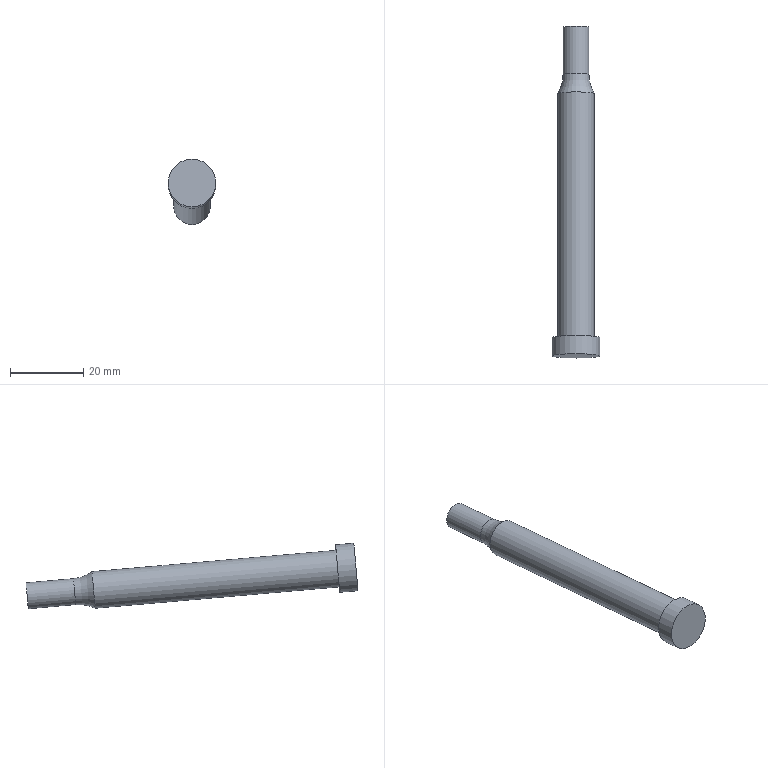Part | NX | features SPAS 10-80-7.100 2 | 1 solid | 7 faces | box 13 x 90.533 x 17.856 mm | volume 6692 mm3 | plane 3 | cylinder 3 | torus 1 | commonest cylinder face diameters 7.1 x1 10 x1 13 x1
STEP:
#1=CARTESIAN_POINT('',(-242.835,-53.602,-36.764));
#2=VERTEX_POINT('',#1);
#3=CARTESIAN_POINT('',(-242.835,-53.292,-33.227));
#4=DIRECTION('',(0.,-0.9962,0.08716));
#5=DIRECTION('',(0.,-0.08716,-0.9962));
#6=AXIS2_PLACEMENT_3D('',#3,#4,#5);
#7=CIRCLE('',#6,3.55);
#8=EDGE_CURVE('',#2,#2,#7,.T.);
#9=ORIENTED_EDGE('',*,*,#8,.F.);
#10=EDGE_LOOP('',(#9));
#11=FACE_BOUND('',#10,.T.);
#12=CARTESIAN_POINT('',(-242.835,-53.292,-33.227));
#13=DIRECTION('',(0.,0.9962,-0.08716));
#14=DIRECTION('',(0.,0.08716,0.9962));
#15=AXIS2_PLACEMENT_3D('',#12,#13,#14);
#16=PLANE('',#15);
#17=ADVANCED_FACE('',(#11),#16,.T.);
#18=CARTESIAN_POINT('',(-242.835,-66.552,-35.631));
#19=VERTEX_POINT('',#18);
#20=CARTESIAN_POINT('',(-242.835,-66.243,-32.094));
#21=DIRECTION('',(0.,-0.9962,0.08716));
#22=DIRECTION('',(0.,-0.08716,-0.9962));
#23=AXIS2_PLACEMENT_3D('',#20,#21,#22);
#24=CIRCLE('',#23,3.55);
#25=EDGE_CURVE('',#19,#19,#24,.F.);
#26=ORIENTED_EDGE('',*,*,#25,.T.);
#27=EDGE_LOOP('',(#26));
#28=FACE_BOUND('',#27,.T.);
#29=ORIENTED_EDGE('',*,*,#8,.T.);
#30=EDGE_LOOP('',(#29));
#31=FACE_BOUND('',#30,.T.);
#32=CARTESIAN_POINT('',(-242.835,-53.292,-33.227));
#33=DIRECTION('',(0.,-0.9962,0.08716));
#34=DIRECTION('',(0.,-0.08716,-0.9962));
#35=AXIS2_PLACEMENT_3D('',#32,#33,#34);
#36=CYLINDRICAL_SURFACE('',#35,3.55);
#37=ADVANCED_FACE('',(#28,#31),#36,.T.);
#38=CARTESIAN_POINT('',(-242.835,-137.533,-20.838));
#39=VERTEX_POINT('',#38);
#40=CARTESIAN_POINT('',(-242.835,-137.969,-25.819));
#41=DIRECTION('',(0.,0.9962,-0.08716));
#42=DIRECTION('',(0.,0.08716,0.9962));
#43=AXIS2_PLACEMENT_3D('',#40,#41,#42);
#44=CIRCLE('',#43,5.);
#45=EDGE_CURVE('',#39,#39,#44,.F.);
#46=ORIENTED_EDGE('',*,*,#45,.F.);
#47=EDGE_LOOP('',(#46));
#48=FACE_BOUND('',#47,.T.);
#49=CARTESIAN_POINT('',(-242.835,-71.845,-36.623));
#50=VERTEX_POINT('',#49);
#51=CARTESIAN_POINT('',(-242.835,-71.409,-31.642));
#52=DIRECTION('',(0.,-0.9962,0.08716));
#53=DIRECTION('',(0.,-0.08716,-0.9962));
#54=AXIS2_PLACEMENT_3D('',#51,#52,#53);
#55=CIRCLE('',#54,5.);
#56=EDGE_CURVE('',#50,#50,#55,.T.);
#57=ORIENTED_EDGE('',*,*,#56,.T.);
#58=EDGE_LOOP('',(#57));
#59=FACE_BOUND('',#58,.T.);
#60=CARTESIAN_POINT('',(-242.835,-71.409,-31.642));
#61=DIRECTION('',(0.,-0.9962,0.08716));
#62=DIRECTION('',(0.,-0.08716,-0.9962));
#63=AXIS2_PLACEMENT_3D('',#60,#61,#62);
#64=CYLINDRICAL_SURFACE('',#63,5.);
#65=ADVANCED_FACE('',(#48,#59),#64,.T.);
#66=CARTESIAN_POINT('',(-242.835,-143.516,-31.859));
#67=VERTEX_POINT('',#66);
#68=CARTESIAN_POINT('',(-242.835,-142.95,-25.383));
#69=DIRECTION('',(0.,-0.9962,0.08716));
#70=DIRECTION('',(0.,-0.08716,-0.9962));
#71=AXIS2_PLACEMENT_3D('',#68,#69,#70);
#72=CIRCLE('',#71,6.5);
#73=EDGE_CURVE('',#67,#67,#72,.F.);
#74=ORIENTED_EDGE('',*,*,#73,.F.);
#75=EDGE_LOOP('',(#74));
#76=FACE_BOUND('',#75,.T.);
#77=CARTESIAN_POINT('',(-242.835,-142.95,-25.383));
#78=DIRECTION('',(0.,-0.9962,0.08716));
#79=DIRECTION('',(0.,-0.08716,-0.9962));
#80=AXIS2_PLACEMENT_3D('',#77,#78,#79);
#81=PLANE('',#80);
#82=ADVANCED_FACE('',(#76),#81,.T.);
#83=ORIENTED_EDGE('',*,*,#45,.T.);
#84=EDGE_LOOP('',(#83));
#85=FACE_BOUND('',#84,.T.);
#86=CARTESIAN_POINT('',(-242.835,-137.402,-19.344));
#87=VERTEX_POINT('',#86);
#88=CARTESIAN_POINT('',(-242.835,-137.969,-25.819));
#89=DIRECTION('',(0.,0.9962,-0.08716));
#90=DIRECTION('',(0.,0.08716,0.9962));
#91=AXIS2_PLACEMENT_3D('',#88,#89,#90);
#92=CIRCLE('',#91,6.5);
#93=EDGE_CURVE('',#87,#87,#92,.F.);
#94=ORIENTED_EDGE('',*,*,#93,.F.);
#95=EDGE_LOOP('',(#94));
#96=FACE_BOUND('',#95,.T.);
#97=CARTESIAN_POINT('',(-242.835,-137.969,-25.819));
#98=DIRECTION('',(0.,0.9962,-0.08716));
#99=DIRECTION('',(0.,0.08716,0.9962));
#100=AXIS2_PLACEMENT_3D('',#97,#98,#99);
#101=PLANE('',#100);
#102=ADVANCED_FACE('',(#85,#96),#101,.T.);
#103=ORIENTED_EDGE('',*,*,#73,.T.);
#104=EDGE_LOOP('',(#103));
#105=FACE_BOUND('',#104,.T.);
#106=ORIENTED_EDGE('',*,*,#93,.T.);
#107=EDGE_LOOP('',(#106));
#108=FACE_BOUND('',#107,.T.);
#109=CARTESIAN_POINT('',(-242.835,-128.007,-26.691));
#110=DIRECTION('',(0.,-0.9962,0.08716));
#111=DIRECTION('',(0.,-0.08716,-0.9962));
#112=AXIS2_PLACEMENT_3D('',#109,#110,#111);
#113=CYLINDRICAL_SURFACE('',#112,6.5);
#114=ADVANCED_FACE('',(#105,#108),#113,.T.);
#115=ORIENTED_EDGE('',*,*,#25,.F.);
#116=EDGE_LOOP('',(#115));
#117=FACE_BOUND('',#116,.T.);
#118=ORIENTED_EDGE('',*,*,#56,.F.);
#119=EDGE_LOOP('',(#118));
#120=FACE_BOUND('',#119,.T.);
#121=CARTESIAN_POINT('',(-242.835,-66.243,-32.094));
#122=DIRECTION('',(0.,-0.9962,0.08716));
#123=DIRECTION('',(0.,-0.08716,-0.9962));
#124=AXIS2_PLACEMENT_3D('',#121,#122,#123);
#125=TOROIDAL_SURFACE('',#124,13.55,10.);
#126=ADVANCED_FACE('',(#117,#120),#125,.F.);
#127=CLOSED_SHELL('',(#17,#37,#65,#82,#102,#114,#126));
#128=MANIFOLD_SOLID_BREP('',#127);
#129=(LENGTH_UNIT()NAMED_UNIT(*)SI_UNIT(.MILLI.,.METRE.));
#130=UNCERTAINTY_MEASURE_WITH_UNIT(LENGTH_MEASURE(0.00001),#129,'','');
#131=(NAMED_UNIT(*)PLANE_ANGLE_UNIT()SI_UNIT($,.RADIAN.));
#132=(NAMED_UNIT(*)SI_UNIT($,.STERADIAN.)SOLID_ANGLE_UNIT());
#133=(GEOMETRIC_REPRESENTATION_CONTEXT(3)GLOBAL_UNCERTAINTY_ASSIGNED_CONTEXT((#130))GLOBAL_UNIT_ASSIGNED_CONTEXT((#129,#131,#132))REPRESENTATION_CONTEXT('',''));
#134=ADVANCED_BREP_SHAPE_REPRESENTATION('',(#128),#133);